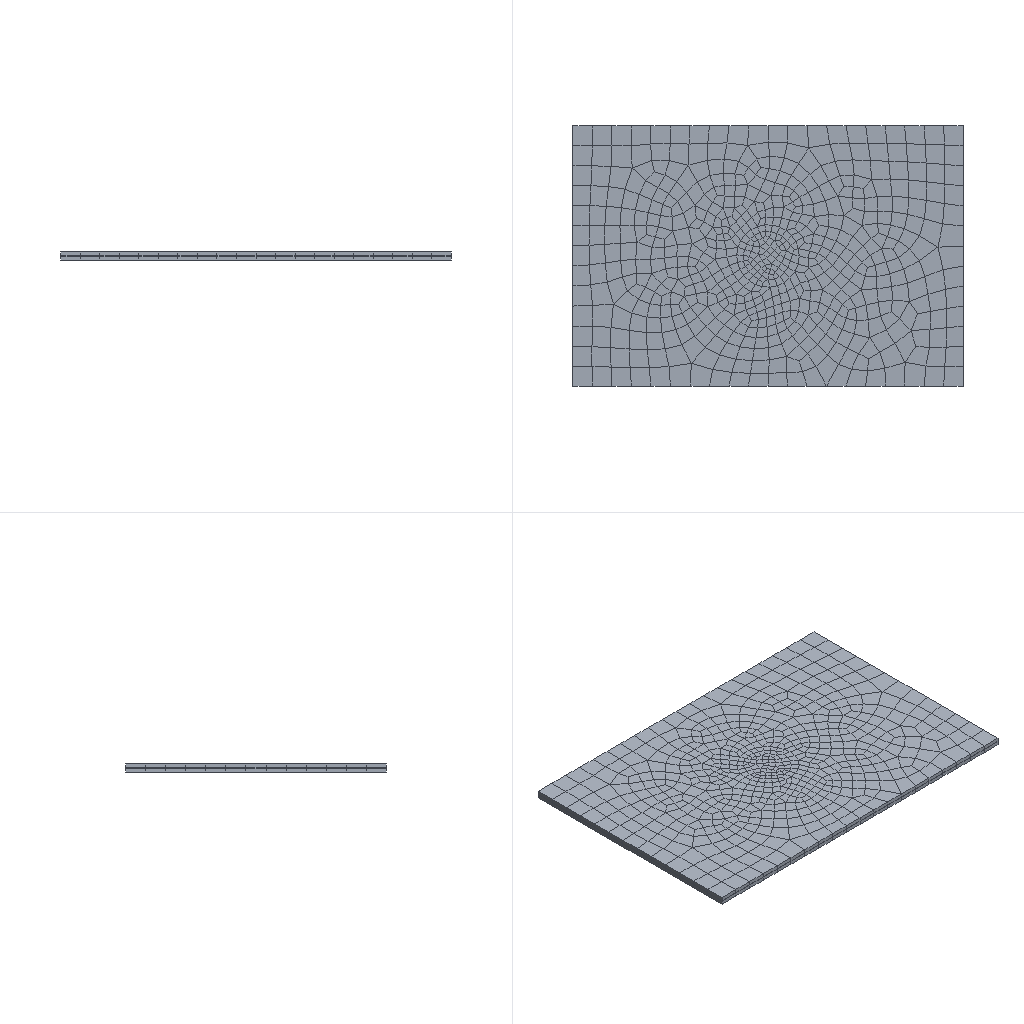Simulation study | abaqus
Set-up summary:
category,name,step,type,value,unit,region
solver,abaqus
solver,version,,,Abaqus/Explicit 2020
units,not stated in the deck,,not stated
analysis,deck,,transient,transient
load_step,Step-1,Step-1,transient
load_step,requested,,,1
mesh,nodes,,,4248
mesh,elements,,,2174
element_type,R3D3,,rigid,6
element_type,R3D4,,rigid,298
element_type,SC8R,,solid_shell,613
element_type,C3D8R,,solid,646
element_type,COH3D8,,cohesive,611
load,load commands in deck,,count,1
bc,support commands in deck,,count,7
material,CFRP,,in results
material,COH,,in results
material,MG,,in results
check,setup vs results,,match,"per instance, exact: element labels, types and connectivity; labels of the nodes the elements use; coordinates of those nodes at SINGLE_PRECISION in 2 of 4 instance(s)"
Abaqus input file, long lists of numbers shortened:
*Heading
** Job name: Job-1 Model name: Model-1
** Generated by: Abaqus/CAE 2020
*Preprint, echo=NO, model=NO, history=NO, contact=NO
**
** PARTS
**
*Part, name=Mg
*Node
      1,           0.,           0.,           0.
      2,         150.,           0.,           0.
** (1358 more lines like these left out)
*Element, type=C3D8R
  1,  190,  204,   77,   76,  709,  723,  166,  165
  2,  216,  202,  214,  240,  735,  721,  733,  759
** (644 more lines like these left out)
*Nset, nset=Set-1, generate
    1,  1360,     1
*Elset, elset=Set-1, generate
   1,  646,    1
** Section: mg
*Solid Section, elset=Set-1, material=mg
,
*End Part
**
*Part, name=cfrp
*Node
      1,           0.,           0.,           0.
      2,         150.,           0.,           0.
** (1292 more lines like these left out)
*Element, type=SC8R
  1,   77,   76,  201,  196,  166,  165,  685,  680
  2,  300,  262,  253,  279,  784,  746,  737,  763
** (611 more lines like these left out)
*Nset, nset=Set-1, generate
    1,  1294,     1
*Elset, elset=Set-1, generate
   1,  613,    1
** Section: cfrpaa
*Shell Section, elset=Set-1, material=cfrp
1., 5
*End Part
**
*Part, name=coh
*Node
      1,         150.,        -100.,  0.1
      2,         150.,           0.,  0.1
** (1288 more lines like these left out)
*Element, type=COH3D8
  1,   83,  206,  224,   84,  173,  692,  710,  174
  2,   80,  198,  219,   81,  170,  684,  705,  171
** (609 more lines like these left out)
*Nset, nset=Set-1, generate
    1,  1290,     1
*Elset, elset=Set-1, generate
   1,  611,    1
** Section: coh
*Cohesive Section, elset=Set-1, controls=EC-1, material=coh, response=TRACTION SEPARATION, thickness=SPECIFIED
0.1,
*End Part
**
*Part, name=rigid
*Node
      1,   5.657,  -5.657,          20.
      2,   5.657,  -5.657,           0.
** (301 more lines like these left out)
*Element, type=R3D4
  1,   1,   3,  45,  66
  2,   3,   4,  46,  45
** (296 more lines like these left out)
*Element, type=R3D3
199, 238,   4,   3
200, 226, 244, 228
** (4 more lines like these left out)
*Node
    304,           0., -4.89858741e-16,          20.
*Nset, nset=rigid-RefPt_, internal
304,
*Elset, elset=rigid, generate
   1,  304,    1
*End Part
**
**
** ASSEMBLY
**
*Assembly, name=Assembly
**
*Instance, name=Mg-1, part=Mg
          0.,           0.,          1.5
*End Instance
**
*Instance, name=cfrp-1, part=cfrp
          0.,           0.,          3.1
*End Instance
**
*Instance, name=coh-1, part=coh
          0.,           0.,           3.
*End Instance
**
*Instance, name=rigid-1, part=rigid
         75.,         -50.,          5.6
*End Instance
**
*Nset, nset=Set-1, instance=Mg-1
   1,   2,   3,   4,   7,   8,   9,  10,  12,  13,  14,  15,  16,  17,  18,  19
  20,  21,  22,  23,  24,  25,  26,  27,  28,  29,  30,  31,  32,  33,  34,  35
** (7 more lines like these left out)
*Nset, nset=Set-1, instance=cfrp-1
   1,   2,   3,   4,   7,   8,   9,  10,  12,  13,  14,  15,  16,  17,  18,  19
  20,  21,  22,  23,  24,  25,  26,  27,  28,  29,  30,  31,  32,  33,  34,  35
** (7 more lines like these left out)
*Nset, nset=Set-1, instance=coh-1
   1,   2,   3,   4,   7,   8,   9,  10,  12,  13,  14,  15,  16,  17,  18,  19
  20,  21,  22,  23,  24,  25,  26,  27,  28,  29,  30,  31,  32,  33,  34,  35
** (7 more lines like these left out)
*Elset, elset=Set-1, instance=Mg-1
   6,  19,  20,  37,  38,  39,  48,  49,  63,  71, 218, 311, 347, 366, 384, 387
 388, 391, 395, 405, 407, 409, 413, 418, 422, 426, 431, 433, 435, 438, 440, 441
** (2 more lines like these left out)
*Elset, elset=Set-1, instance=cfrp-1
   5,  19,  34,  35,  45,  46,  59,  60,  67, 175, 221, 267, 274, 284, 292, 318
 319, 333, 344, 349, 351, 352, 363, 376, 378, 379, 383, 392, 400, 402, 404, 405
** (2 more lines like these left out)
*Elset, elset=Set-1, instance=coh-1
  11,  18,  19,  30,  31,  32,  46,  47,  48,  57,  58,  59,  71, 220, 235, 248
 249, 279, 282, 283, 287, 288, 300, 309, 310, 313, 314, 320, 323, 330, 333, 334
** (2 more lines like these left out)
*Nset, nset=Set-3, instance=rigid-1
 304,
*Nset, nset=s_Set-2, instance=Mg-1
    5,    6,   11,   74,   75,   76,   77,   78,   79,   80,   81,   82,   83,   84,   85,   86
   87,   88,   89,   90,   91,   92,   93,   94,   95,   96,   97,  160,  161,  162,  163,  164
** (10 more lines like these left out)
*Nset, nset=s_Set-2, instance=cfrp-1
    5,    6,   11,   74,   75,   76,   77,   78,   79,   80,   81,   82,   83,   84,   85,   86
   87,   88,   89,   90,   91,   92,   93,   94,   95,   96,   97,  160,  161,  162,  163,  164
** (11 more lines like these left out)
*Nset, nset=s_Set-2, instance=coh-1
    5,    6,   11,   74,   75,   76,   77,   78,   79,   80,   81,   82,   83,   84,   85,   86
   87,   88,   89,   90,   91,   92,   93,   94,   95,   96,   97,  160,  161,  162,  163,  164
** (10 more lines like these left out)
*Elset, elset=s_Set-2, instance=Mg-1, generate
 566,  646,    1
*Elset, elset=s_Set-2, instance=cfrp-1, generate
 531,  613,    1
*Elset, elset=s_Set-2, instance=coh-1, generate
 533,  611,    1
*Nset, nset=s_Set-4, instance=cfrp-1
    5,    6,   11,   74,   75,   76,   77,   78,   79,   80,   81,   82,   83,   84,   85,   86
   87,   88,   89,   90,   91,   92,   93,   94,   95,   96,   97,  160,  161,  162,  163,  164
** (11 more lines like these left out)
*Elset, elset=s_Set-4, instance=cfrp-1, generate
 531,  613,    1
*Nset, nset=s_Set-5, instance=coh-1
    5,    6,   11,   74,   75,   76,   77,   78,   79,   80,   81,   82,   83,   84,   85,   86
   87,   88,   89,   90,   91,   92,   93,   94,   95,   96,   97,  160,  161,  162,  163,  164
** (10 more lines like these left out)
*Elset, elset=s_Set-5, instance=coh-1, generate
 533,  611,    1
*Nset, nset=s_Set-6, instance=Mg-1
    5,    6,   11,   74,   75,   76,   77,   78,   79,   80,   81,   82,   83,   84,   85,   86
   87,   88,   89,   90,   91,   92,   93,   94,   95,   96,   97,  160,  161,  162,  163,  164
** (10 more lines like these left out)
*Elset, elset=s_Set-6, instance=Mg-1, generate
 566,  646,    1
*Elset, elset=_m_Surf-1_S1, internal, instance=cfrp-1, generate
   1,  530,    1
*Elset, elset=_m_Surf-1_S2, internal, instance=cfrp-1, generate
 531,  613,    1
*Surface, type=ELEMENT, name=m_Surf-1
_m_Surf-1_S1, S1
_m_Surf-1_S2, S2
*Elset, elset=_m_Surf-3_S2, internal, instance=coh-1, generate
   1,  532,    1
*Elset, elset=_m_Surf-3_S1, internal, instance=coh-1, generate
 533,  611,    1
*Surface, type=ELEMENT, name=m_Surf-3
_m_Surf-3_S2, S2
_m_Surf-3_S1, S1
*Elset, elset=_m_Surf-5_SPOS, internal, instance=rigid-1, generate
   1,  304,    1
*Surface, type=ELEMENT, name=m_Surf-5
_m_Surf-5_SPOS, SPOS
*Elset, elset=_s_Surf-1_S1, internal, instance=coh-1, generate
   1,  532,    1
*Elset, elset=_s_Surf-1_S2, internal, instance=coh-1, generate
 533,  611,    1
*Surface, type=ELEMENT, name=s_Surf-1
_s_Surf-1_S1, S1
_s_Surf-1_S2, S2
*Elset, elset=_s_Surf-3_S2, internal, instance=Mg-1, generate
   1,  565,    1
*Elset, elset=_s_Surf-3_S1, internal, instance=Mg-1, generate
 566,  646,    1
*Surface, type=ELEMENT, name=s_Surf-3
_s_Surf-3_S2, S2
_s_Surf-3_S1, S1
*Rigid Body, ref node=rigid-1.rigid-RefPt_, elset=rigid-1.rigid
** Constraint: Constraint-1
*Tie, name=Constraint-1, adjust=yes
s_Surf-1, m_Surf-1
** Constraint: Constraint-2
*Tie, name=Constraint-2, adjust=yes
s_Surf-3, m_Surf-3
*End Assembly
**
** ELEMENT CONTROLS
**
*Section Controls, name=EC-1, ELEMENT DELETION=YES
1., 1., 1.
**
** MATERIALS
**
*Material, name=cfrp
*Damage Initiation, criterion=HASHIN
100.,157., 29., 36., 67., 67.
*Damage Evolution, type=ENERGY
2000.,2000.,2000.,2000.
*Density
 2e-09,
*Elastic, type=LAMINA
131000.,9000.,  0.3,5000.,5000.,5000.
*Material, name=coh
*Damage Initiation, criterion=QUADE
 0.04, 0.04, 0.04
*Damage Evolution, type=DISPLACEMENT
 1e-19,
*Density
 1.5e-09,
*Elastic, type=TRACTION
10000.,8000.,8000.
*Material, name=mg
*Damage Initiation, criterion=SHEAR
 0.1,0.,0.
*Damage Evolution, type=DISPLACEMENT
 0.0001,
*Density
 1.74e-09,
*Elastic
45000., 0.34
*Plastic
300.,0.
**
** INTERACTION PROPERTIES
**
*Surface Interaction, name=IntProp-1
*Friction
 0.2,
*Surface Behavior, pressure-overclosure=HARD
** ----------------------------------------------------------------
**
** STEP: Step-1
**
*Step, name=Step-1, nlgeom=YES
*Dynamic, Explicit
, 0.015
*Bulk Viscosity
0.06, 1.2
** Mass Scaling: Semi-Automatic
**               Whole Model
*Fixed Mass Scaling, factor=500.
**
** BOUNDARY CONDITIONS
**
** Name: BC-1 Type: 对称/反对称/完全固定
*Boundary
Set-1, ENCASTRE
** Name: BC-2 Type: 速度/角速度
*Boundary, type=VELOCITY
Set-3, 1, 1
Set-3, 2, 2
Set-3, 3, 3, -1000.
Set-3, 4, 4
Set-3, 5, 5
Set-3, 6, 6
**
** INTERACTIONS
**
** Interaction: Int-4
*Contact, op=NEW
*Contact Inclusions, ALL EXTERIOR
*Contact Property Assignment
 ,  , IntProp-1
**
** OUTPUT REQUESTS
**
*Restart, write, number interval=1, time marks=NO
**
** FIELD OUTPUT: F-Output-1
**
*Output, field, number interval=50
*Node Output
A, CF, RF, RM, RT, U, V
*Element Output, directions=YES
DAMAGEFC, DAMAGEFT, DAMAGEMC, DAMAGEMT, E, EVF, LE, MISES, MISESMAX, PE, PEEQ, PEEQVAVG, PEVAVG, S, SDEG, SF
STATUS, SVAVG
*Contact Output
CDISP, CFORCE, CSDMG, CSTRESS
**
** HISTORY OUTPUT: H-Output-1
**
*Output, history, time interval=7.5e-06
*Node Output, nset=Set-3
RF1, RF2, RF3
*End Step
Results summary:
result,step,Step-1,completed,increments=53077 time=0.015/0.015
result,analysis,,,transient
result,last_loadstep,,,1
result,primary field,,,U
result,reaction total,,FX,2494.275,model units
result,reaction total,,FY,-5240.611,model units
result,reaction total,,FZ,-44510.016,model units